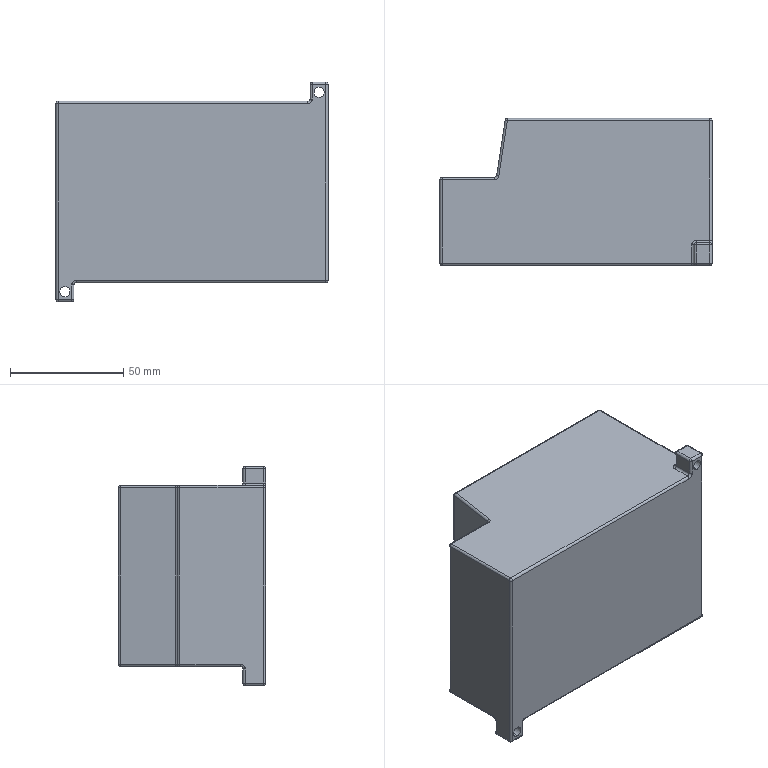Part | STEP file | IO expansion module HCB2-1616-DTD01 | 1 solid | 78 faces | box 120.4 x 65 x 97 mm | volume 571916 mm3 | cylinder 40 | sphere 16 | plane 14 | torus 8 | commonest cylinder face diameters 2 x36 4.5 x4